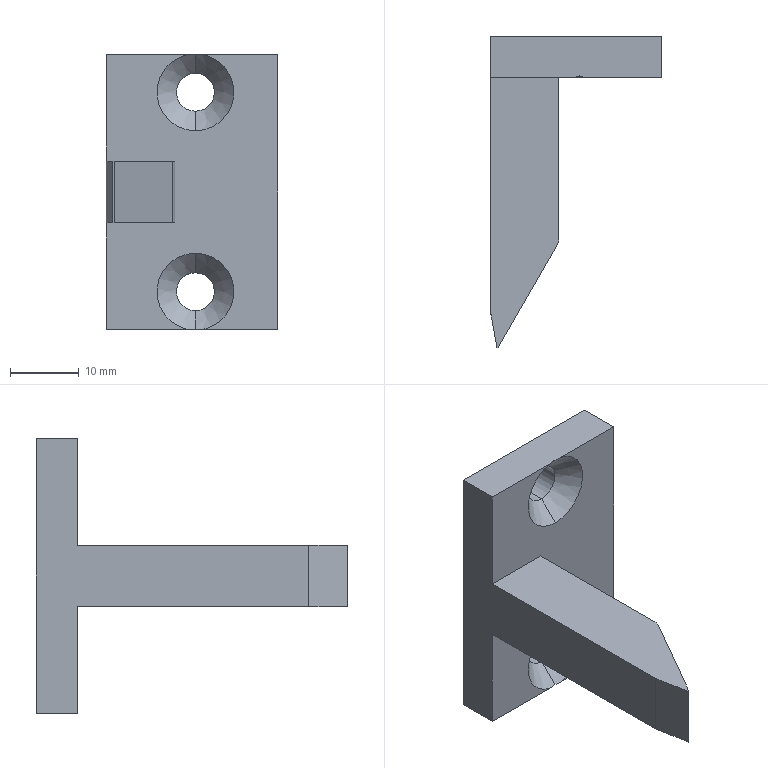Part | STEP file | PN_0002NACCTV wedge pin 527 | 1 solid | 21 faces | box 25 x 45.321 x 40 mm | volume 8429 mm3 | plane 12 | cylinder 5 | cone 4 | commonest cylinder face diameters 5.5 x4 4 x1
STEP:
#1=CARTESIAN_POINT('',(4.4,39.275,-11.75));
#2=VERTEX_POINT('',#1);
#3=CARTESIAN_POINT('',(4.4,39.275,-17.25));
#4=VERTEX_POINT('',#3);
#5=CARTESIAN_POINT('',(4.4,39.275,-14.5));
#6=DIRECTION('',(0.,-1.,0.));
#7=DIRECTION('',(0.,0.,-1.));
#8=AXIS2_PLACEMENT_3D('',#5,#6,#7);
#9=CIRCLE('',#8,2.75);
#10=EDGE_CURVE('',#2,#4,#9,.T.);
#11=ORIENTED_EDGE('',*,*,#10,.F.);
#12=CARTESIAN_POINT('',(4.4,36.425,-8.9));
#13=VERTEX_POINT('',#12);
#14=CARTESIAN_POINT('',(4.4,36.425,-8.9));
#15=DIRECTION('',(0.,-0.7071,0.7071));
#16=VECTOR('',#15,1000.);
#17=LINE('',#14,#16);
#18=EDGE_CURVE('',#2,#13,#17,.T.);
#19=ORIENTED_EDGE('',*,*,#18,.T.);
#20=CARTESIAN_POINT('',(3.346,36.425,-20.));
#21=VERTEX_POINT('',#20);
#22=CARTESIAN_POINT('',(4.4,36.425,-14.5));
#23=DIRECTION('',(0.,-1.,0.));
#24=DIRECTION('',(0.,0.,-1.));
#25=AXIS2_PLACEMENT_3D('',#22,#23,#24);
#26=CIRCLE('',#25,5.6);
#27=EDGE_CURVE('',#13,#21,#26,.T.);
#28=ORIENTED_EDGE('',*,*,#27,.T.);
#29=CARTESIAN_POINT('',(4.4,36.525,-20.));
#30=VERTEX_POINT('',#29);
#31=CARTESIAN_POINT('',(3.346,36.425,-20.));
#32=CARTESIAN_POINT('',(3.695,36.491,-20.));
#33=CARTESIAN_POINT('',(4.047,36.525,-20.));
#34=CARTESIAN_POINT('',(4.4,36.525,-20.));
#35=B_SPLINE_CURVE_WITH_KNOTS('',3,(#31,#32,#33,#34),.UNSPECIFIED.,.F.,.F.,(4,4),(0.01324,0.01428),.UNSPECIFIED.);
#36=EDGE_CURVE('',#21,#30,#35,.T.);
#37=ORIENTED_EDGE('',*,*,#36,.T.);
#38=CARTESIAN_POINT('',(4.4,36.425,-20.1));
#39=DIRECTION('',(0.,-0.7071,-0.7071));
#40=VECTOR('',#39,1000.);
#41=LINE('',#38,#40);
#42=EDGE_CURVE('',#4,#30,#41,.T.);
#43=ORIENTED_EDGE('',*,*,#42,.F.);
#44=EDGE_LOOP('',(#11,#19,#28,#37,#43));
#45=FACE_OUTER_BOUND('',#44,.T.);
#46=CARTESIAN_POINT('',(4.4,36.425,-14.5));
#47=DIRECTION('',(0.,-1.,0.));
#48=DIRECTION('',(0.,0.,-1.));
#49=AXIS2_PLACEMENT_3D('',#46,#47,#48);
#50=CONICAL_SURFACE('',#49,5.6,0.7854);
#51=ADVANCED_FACE('',(#45),#50,.F.);
#52=CARTESIAN_POINT('',(4.4,42.425,-11.75));
#53=VERTEX_POINT('',#52);
#54=CARTESIAN_POINT('',(4.4,42.425,-17.25));
#55=VERTEX_POINT('',#54);
#56=CARTESIAN_POINT('',(4.4,42.425,-14.5));
#57=DIRECTION('',(0.,-1.,0.));
#58=DIRECTION('',(0.,0.,-1.));
#59=AXIS2_PLACEMENT_3D('',#56,#57,#58);
#60=CIRCLE('',#59,2.75);
#61=EDGE_CURVE('',#53,#55,#60,.T.);
#62=ORIENTED_EDGE('',*,*,#61,.F.);
#63=CARTESIAN_POINT('',(4.4,36.425,-11.75));
#64=DIRECTION('',(0.,-1.,0.));
#65=VECTOR('',#64,1000.);
#66=LINE('',#63,#65);
#67=EDGE_CURVE('',#53,#2,#66,.T.);
#68=ORIENTED_EDGE('',*,*,#67,.T.);
#69=ORIENTED_EDGE('',*,*,#10,.T.);
#70=CARTESIAN_POINT('',(4.4,36.425,-17.25));
#71=DIRECTION('',(0.,-1.,0.));
#72=VECTOR('',#71,1000.);
#73=LINE('',#70,#72);
#74=EDGE_CURVE('',#55,#4,#73,.T.);
#75=ORIENTED_EDGE('',*,*,#74,.F.);
#76=EDGE_LOOP('',(#62,#68,#69,#75));
#77=FACE_OUTER_BOUND('',#76,.T.);
#78=CARTESIAN_POINT('',(4.4,36.425,-14.5));
#79=DIRECTION('',(0.,-1.,0.));
#80=DIRECTION('',(0.,0.,-1.));
#81=AXIS2_PLACEMENT_3D('',#78,#79,#80);
#82=CYLINDRICAL_SURFACE('',#81,2.75);
#83=ADVANCED_FACE('',(#77),#82,.F.);
#84=CARTESIAN_POINT('',(4.4,39.275,17.25));
#85=VERTEX_POINT('',#84);
#86=CARTESIAN_POINT('',(4.4,39.275,11.75));
#87=VERTEX_POINT('',#86);
#88=CARTESIAN_POINT('',(4.4,39.275,14.5));
#89=DIRECTION('',(0.,-1.,0.));
#90=DIRECTION('',(0.,0.,-1.));
#91=AXIS2_PLACEMENT_3D('',#88,#89,#90);
#92=CIRCLE('',#91,2.75);
#93=EDGE_CURVE('',#85,#87,#92,.T.);
#94=ORIENTED_EDGE('',*,*,#93,.F.);
#95=CARTESIAN_POINT('',(4.4,36.525,20.));
#96=VERTEX_POINT('',#95);
#97=CARTESIAN_POINT('',(4.4,36.425,20.1));
#98=DIRECTION('',(0.,-0.7071,0.7071));
#99=VECTOR('',#98,1000.);
#100=LINE('',#97,#99);
#101=EDGE_CURVE('',#85,#96,#100,.T.);
#102=ORIENTED_EDGE('',*,*,#101,.T.);
#103=CARTESIAN_POINT('',(3.346,36.425,20.));
#104=VERTEX_POINT('',#103);
#105=CARTESIAN_POINT('',(4.4,36.525,20.));
#106=CARTESIAN_POINT('',(4.047,36.525,20.));
#107=CARTESIAN_POINT('',(3.695,36.491,20.));
#108=CARTESIAN_POINT('',(3.346,36.425,20.));
#109=B_SPLINE_CURVE_WITH_KNOTS('',3,(#105,#106,#107,#108),.UNSPECIFIED.,.F.,.F.,(4,4),(0.007613,0.008661),.UNSPECIFIED.);
#110=EDGE_CURVE('',#96,#104,#109,.T.);
#111=ORIENTED_EDGE('',*,*,#110,.T.);
#112=CARTESIAN_POINT('',(4.4,36.425,8.9));
#113=VERTEX_POINT('',#112);
#114=CARTESIAN_POINT('',(4.4,36.425,14.5));
#115=DIRECTION('',(0.,-1.,0.));
#116=DIRECTION('',(0.,0.,-1.));
#117=AXIS2_PLACEMENT_3D('',#114,#115,#116);
#118=CIRCLE('',#117,5.6);
#119=EDGE_CURVE('',#104,#113,#118,.T.);
#120=ORIENTED_EDGE('',*,*,#119,.T.);
#121=CARTESIAN_POINT('',(4.4,36.425,8.9));
#122=DIRECTION('',(0.,-0.7071,-0.7071));
#123=VECTOR('',#122,1000.);
#124=LINE('',#121,#123);
#125=EDGE_CURVE('',#87,#113,#124,.T.);
#126=ORIENTED_EDGE('',*,*,#125,.F.);
#127=EDGE_LOOP('',(#94,#102,#111,#120,#126));
#128=FACE_OUTER_BOUND('',#127,.T.);
#129=CARTESIAN_POINT('',(4.4,36.425,14.5));
#130=DIRECTION('',(0.,-1.,0.));
#131=DIRECTION('',(0.,0.,-1.));
#132=AXIS2_PLACEMENT_3D('',#129,#130,#131);
#133=CONICAL_SURFACE('',#132,5.6,0.7854);
#134=ADVANCED_FACE('',(#128),#133,.F.);
#135=CARTESIAN_POINT('',(4.4,42.425,17.25));
#136=VERTEX_POINT('',#135);
#137=CARTESIAN_POINT('',(4.4,42.425,11.75));
#138=VERTEX_POINT('',#137);
#139=CARTESIAN_POINT('',(4.4,42.425,14.5));
#140=DIRECTION('',(0.,-1.,0.));
#141=DIRECTION('',(0.,0.,-1.));
#142=AXIS2_PLACEMENT_3D('',#139,#140,#141);
#143=CIRCLE('',#142,2.75);
#144=EDGE_CURVE('',#136,#138,#143,.T.);
#145=ORIENTED_EDGE('',*,*,#144,.F.);
#146=CARTESIAN_POINT('',(4.4,36.425,17.25));
#147=DIRECTION('',(0.,-1.,0.));
#148=VECTOR('',#147,1000.);
#149=LINE('',#146,#148);
#150=EDGE_CURVE('',#136,#85,#149,.T.);
#151=ORIENTED_EDGE('',*,*,#150,.T.);
#152=ORIENTED_EDGE('',*,*,#93,.T.);
#153=CARTESIAN_POINT('',(4.4,36.425,11.75));
#154=DIRECTION('',(0.,-1.,0.));
#155=VECTOR('',#154,1000.);
#156=LINE('',#153,#155);
#157=EDGE_CURVE('',#138,#87,#156,.T.);
#158=ORIENTED_EDGE('',*,*,#157,.F.);
#159=EDGE_LOOP('',(#145,#151,#152,#158));
#160=FACE_OUTER_BOUND('',#159,.T.);
#161=CARTESIAN_POINT('',(4.4,36.425,14.5));
#162=DIRECTION('',(0.,-1.,0.));
#163=DIRECTION('',(0.,0.,-1.));
#164=AXIS2_PLACEMENT_3D('',#161,#162,#163);
#165=CYLINDRICAL_SURFACE('',#164,2.75);
#166=ADVANCED_FACE('',(#160),#165,.F.);
#167=CARTESIAN_POINT('',(-8.6,42.425,20.));
#168=VERTEX_POINT('',#167);
#169=CARTESIAN_POINT('',(-8.6,42.425,-20.));
#170=VERTEX_POINT('',#169);
#171=CARTESIAN_POINT('',(-8.6,42.425,4.5));
#172=DIRECTION('',(0.,0.,-1.));
#173=VECTOR('',#172,1000.);
#174=LINE('',#171,#173);
#175=EDGE_CURVE('',#168,#170,#174,.T.);
#176=ORIENTED_EDGE('',*,*,#175,.T.);
#177=CARTESIAN_POINT('',(-8.6,36.425,-20.));
#178=VERTEX_POINT('',#177);
#179=CARTESIAN_POINT('',(-8.6,36.425,-20.));
#180=DIRECTION('',(0.,1.,0.));
#181=VECTOR('',#180,1000.);
#182=LINE('',#179,#181);
#183=EDGE_CURVE('',#178,#170,#182,.T.);
#184=ORIENTED_EDGE('',*,*,#183,.F.);
#185=CARTESIAN_POINT('',(-8.6,36.425,-4.5));
#186=VERTEX_POINT('',#185);
#187=CARTESIAN_POINT('',(-8.6,36.425,-20.));
#188=DIRECTION('',(0.,0.,1.));
#189=VECTOR('',#188,1000.);
#190=LINE('',#187,#189);
#191=EDGE_CURVE('',#178,#186,#190,.T.);
#192=ORIENTED_EDGE('',*,*,#191,.T.);
#193=CARTESIAN_POINT('',(-8.6,2.776,-4.5));
#194=VERTEX_POINT('',#193);
#195=CARTESIAN_POINT('',(-8.6,-4.896,-4.5));
#196=DIRECTION('',(0.,-1.,0.));
#197=VECTOR('',#196,1000.);
#198=LINE('',#195,#197);
#199=EDGE_CURVE('',#186,#194,#198,.T.);
#200=ORIENTED_EDGE('',*,*,#199,.T.);
#201=CARTESIAN_POINT('',(-8.6,2.776,4.5));
#202=VERTEX_POINT('',#201);
#203=CARTESIAN_POINT('',(-8.6,2.776,4.5));
#204=DIRECTION('',(0.,0.,1.));
#205=VECTOR('',#204,1000.);
#206=LINE('',#203,#205);
#207=EDGE_CURVE('',#194,#202,#206,.T.);
#208=ORIENTED_EDGE('',*,*,#207,.T.);
#209=CARTESIAN_POINT('',(-8.6,36.425,4.5));
#210=VERTEX_POINT('',#209);
#211=CARTESIAN_POINT('',(-8.6,-4.896,4.5));
#212=DIRECTION('',(0.,-1.,0.));
#213=VECTOR('',#212,1000.);
#214=LINE('',#211,#213);
#215=EDGE_CURVE('',#210,#202,#214,.T.);
#216=ORIENTED_EDGE('',*,*,#215,.F.);
#217=CARTESIAN_POINT('',(-8.6,36.425,20.));
#218=VERTEX_POINT('',#217);
#219=CARTESIAN_POINT('',(-8.6,36.425,4.5));
#220=DIRECTION('',(0.,0.,1.));
#221=VECTOR('',#220,1000.);
#222=LINE('',#219,#221);
#223=EDGE_CURVE('',#210,#218,#222,.T.);
#224=ORIENTED_EDGE('',*,*,#223,.T.);
#225=CARTESIAN_POINT('',(-8.6,36.425,20.));
#226=DIRECTION('',(0.,1.,0.));
#227=VECTOR('',#226,1000.);
#228=LINE('',#225,#227);
#229=EDGE_CURVE('',#218,#168,#228,.T.);
#230=ORIENTED_EDGE('',*,*,#229,.T.);
#231=EDGE_LOOP('',(#176,#184,#192,#200,#208,#216,#224,#230));
#232=FACE_OUTER_BOUND('',#231,.T.);
#233=CARTESIAN_POINT('',(-8.6,-4.896,4.5));
#234=DIRECTION('',(1.,0.,0.));
#235=DIRECTION('',(0.,0.,-1.));
#236=AXIS2_PLACEMENT_3D('',#233,#234,#235);
#237=PLANE('',#236);
#238=ADVANCED_FACE('',(#232),#237,.F.);
#239=CARTESIAN_POINT('',(-7.445,-2.896,-4.5));
#240=VERTEX_POINT('',#239);
#241=CARTESIAN_POINT('',(1.132,11.961,-4.5));
#242=VERTEX_POINT('',#241);
#243=CARTESIAN_POINT('',(-8.6,-4.896,-4.5));
#244=DIRECTION('',(0.5,0.866,0.));
#245=VECTOR('',#244,1000.);
#246=LINE('',#243,#245);
#247=EDGE_CURVE('',#240,#242,#246,.T.);
#248=ORIENTED_EDGE('',*,*,#247,.T.);
#249=CARTESIAN_POINT('',(1.132,11.961,4.5));
#250=VERTEX_POINT('',#249);
#251=CARTESIAN_POINT('',(1.132,11.961,4.5));
#252=DIRECTION('',(0.,0.,1.));
#253=VECTOR('',#252,1000.);
#254=LINE('',#251,#253);
#255=EDGE_CURVE('',#242,#250,#254,.T.);
#256=ORIENTED_EDGE('',*,*,#255,.T.);
#257=CARTESIAN_POINT('',(-7.445,-2.896,4.5));
#258=VERTEX_POINT('',#257);
#259=CARTESIAN_POINT('',(-8.6,-4.896,4.5));
#260=DIRECTION('',(0.5,0.866,0.));
#261=VECTOR('',#260,1000.);
#262=LINE('',#259,#261);
#263=EDGE_CURVE('',#258,#250,#262,.T.);
#264=ORIENTED_EDGE('',*,*,#263,.F.);
#265=CARTESIAN_POINT('',(-7.445,-2.896,-4.5));
#266=DIRECTION('',(0.,0.,1.));
#267=VECTOR('',#266,1000.);
#268=LINE('',#265,#267);
#269=EDGE_CURVE('',#240,#258,#268,.T.);
#270=ORIENTED_EDGE('',*,*,#269,.F.);
#271=EDGE_LOOP('',(#248,#256,#264,#270));
#272=FACE_OUTER_BOUND('',#271,.T.);
#273=CARTESIAN_POINT('',(-8.6,-4.896,4.5));
#274=DIRECTION('',(-0.866,0.5,0.));
#275=DIRECTION('',(-0.5,-0.866,0.));
#276=AXIS2_PLACEMENT_3D('',#273,#274,#275);
#277=PLANE('',#276);
#278=ADVANCED_FACE('',(#272),#277,.F.);
#279=CARTESIAN_POINT('',(1.4,12.961,-4.5));
#280=VERTEX_POINT('',#279);
#281=CARTESIAN_POINT('',(1.4,36.425,-4.5));
#282=VERTEX_POINT('',#281);
#283=CARTESIAN_POINT('',(1.4,42.425,-4.5));
#284=DIRECTION('',(0.,1.,0.));
#285=VECTOR('',#284,1000.);
#286=LINE('',#283,#285);
#287=EDGE_CURVE('',#280,#282,#286,.T.);
#288=ORIENTED_EDGE('',*,*,#287,.T.);
#289=CARTESIAN_POINT('',(1.4,36.425,4.5));
#290=VERTEX_POINT('',#289);
#291=CARTESIAN_POINT('',(1.4,36.425,-4.5));
#292=DIRECTION('',(0.,0.,1.));
#293=VECTOR('',#292,1000.);
#294=LINE('',#291,#293);
#295=EDGE_CURVE('',#282,#290,#294,.T.);
#296=ORIENTED_EDGE('',*,*,#295,.T.);
#297=CARTESIAN_POINT('',(1.4,12.961,4.5));
#298=VERTEX_POINT('',#297);
#299=CARTESIAN_POINT('',(1.4,42.425,4.5));
#300=DIRECTION('',(0.,1.,0.));
#301=VECTOR('',#300,1000.);
#302=LINE('',#299,#301);
#303=EDGE_CURVE('',#298,#290,#302,.T.);
#304=ORIENTED_EDGE('',*,*,#303,.F.);
#305=CARTESIAN_POINT('',(1.4,12.961,4.5));
#306=DIRECTION('',(0.,0.,-1.));
#307=VECTOR('',#306,1000.);
#308=LINE('',#305,#307);
#309=EDGE_CURVE('',#298,#280,#308,.T.);
#310=ORIENTED_EDGE('',*,*,#309,.T.);
#311=EDGE_LOOP('',(#288,#296,#304,#310));
#312=FACE_OUTER_BOUND('',#311,.T.);
#313=CARTESIAN_POINT('',(1.4,42.425,4.5));
#314=DIRECTION('',(-1.,0.,0.));
#315=DIRECTION('',(0.,-1.,0.));
#316=AXIS2_PLACEMENT_3D('',#313,#314,#315);
#317=PLANE('',#316);
#318=ADVANCED_FACE('',(#312),#317,.F.);
#319=CARTESIAN_POINT('',(4.4,42.425,-14.5));
#320=DIRECTION('',(0.,-1.,0.));
#321=DIRECTION('',(0.,0.,-1.));
#322=AXIS2_PLACEMENT_3D('',#319,#320,#321);
#323=CIRCLE('',#322,2.75);
#324=EDGE_CURVE('',#55,#53,#323,.T.);
#325=ORIENTED_EDGE('',*,*,#324,.T.);
#326=ORIENTED_EDGE('',*,*,#61,.T.);
#327=EDGE_LOOP('',(#325,#326));
#328=FACE_BOUND('',#327,.T.);
#329=CARTESIAN_POINT('',(4.4,42.425,14.5));
#330=DIRECTION('',(0.,-1.,0.));
#331=DIRECTION('',(0.,0.,-1.));
#332=AXIS2_PLACEMENT_3D('',#329,#330,#331);
#333=CIRCLE('',#332,2.75);
#334=EDGE_CURVE('',#138,#136,#333,.T.);
#335=ORIENTED_EDGE('',*,*,#334,.T.);
#336=ORIENTED_EDGE('',*,*,#144,.T.);
#337=EDGE_LOOP('',(#335,#336));
#338=FACE_BOUND('',#337,.T.);
#339=ORIENTED_EDGE('',*,*,#175,.F.);
#340=CARTESIAN_POINT('',(16.4,42.425,20.));
#341=VERTEX_POINT('',#340);
#342=CARTESIAN_POINT('',(16.4,42.425,20.));
#343=DIRECTION('',(1.,0.,0.));
#344=VECTOR('',#343,1000.);
#345=LINE('',#342,#344);
#346=EDGE_CURVE('',#168,#341,#345,.T.);
#347=ORIENTED_EDGE('',*,*,#346,.T.);
#348=CARTESIAN_POINT('',(16.4,42.425,-20.));
#349=VERTEX_POINT('',#348);
#350=CARTESIAN_POINT('',(16.4,42.425,-20.));
#351=DIRECTION('',(0.,0.,-1.));
#352=VECTOR('',#351,1000.);
#353=LINE('',#350,#352);
#354=EDGE_CURVE('',#341,#349,#353,.T.);
#355=ORIENTED_EDGE('',*,*,#354,.T.);
#356=CARTESIAN_POINT('',(16.4,42.425,-20.));
#357=DIRECTION('',(-1.,0.,0.));
#358=VECTOR('',#357,1000.);
#359=LINE('',#356,#358);
#360=EDGE_CURVE('',#349,#170,#359,.T.);
#361=ORIENTED_EDGE('',*,*,#360,.T.);
#362=EDGE_LOOP('',(#339,#347,#355,#361));
#363=FACE_OUTER_BOUND('',#362,.T.);
#364=CARTESIAN_POINT('',(-8.6,42.425,4.5));
#365=DIRECTION('',(0.,-1.,0.));
#366=DIRECTION('',(0.,0.,-1.));
#367=AXIS2_PLACEMENT_3D('',#364,#365,#366);
#368=PLANE('',#367);
#369=ADVANCED_FACE('',(#328,#338,#363),#368,.F.);
#370=ORIENTED_EDGE('',*,*,#303,.T.);
#371=CARTESIAN_POINT('',(1.4,36.425,4.5));
#372=DIRECTION('',(-1.,0.,0.));
#373=VECTOR('',#372,1000.);
#374=LINE('',#371,#373);
#375=EDGE_CURVE('',#290,#210,#374,.T.);
#376=ORIENTED_EDGE('',*,*,#375,.T.);
#377=ORIENTED_EDGE('',*,*,#215,.T.);
#378=CARTESIAN_POINT('',(-7.6,-2.896,4.5));
#379=VERTEX_POINT('',#378);
#380=CARTESIAN_POINT('',(-8.6,2.776,4.5));
#381=DIRECTION('',(0.1736,-0.9848,0.));
#382=VECTOR('',#381,1000.);
#383=LINE('',#380,#382);
#384=EDGE_CURVE('',#202,#379,#383,.T.);
#385=ORIENTED_EDGE('',*,*,#384,.T.);
#386=CARTESIAN_POINT('',(-8.6,-2.896,4.5));
#387=DIRECTION('',(-1.,0.,0.));
#388=VECTOR('',#387,1000.);
#389=LINE('',#386,#388);
#390=EDGE_CURVE('',#258,#379,#389,.T.);
#391=ORIENTED_EDGE('',*,*,#390,.F.);
#392=ORIENTED_EDGE('',*,*,#263,.T.);
#393=CARTESIAN_POINT('',(-0.6,12.961,4.5));
#394=DIRECTION('',(0.,0.,1.));
#395=DIRECTION('',(-1.,0.,0.));
#396=AXIS2_PLACEMENT_3D('',#393,#394,#395);
#397=CIRCLE('',#396,2.);
#398=EDGE_CURVE('',#250,#298,#397,.T.);
#399=ORIENTED_EDGE('',*,*,#398,.T.);
#400=EDGE_LOOP('',(#370,#376,#377,#385,#391,#392,#399));
#401=FACE_OUTER_BOUND('',#400,.T.);
#402=CARTESIAN_POINT('',(0.,0.,4.5));
#403=DIRECTION('',(0.,0.,-1.));
#404=DIRECTION('',(-1.,0.,0.));
#405=AXIS2_PLACEMENT_3D('',#402,#403,#404);
#406=PLANE('',#405);
#407=ADVANCED_FACE('',(#401),#406,.F.);
#408=CARTESIAN_POINT('',(1.4,36.425,-4.5));
#409=DIRECTION('',(1.,0.,0.));
#410=VECTOR('',#409,1000.);
#411=LINE('',#408,#410);
#412=EDGE_CURVE('',#186,#282,#411,.T.);
#413=ORIENTED_EDGE('',*,*,#412,.T.);
#414=ORIENTED_EDGE('',*,*,#287,.F.);
#415=CARTESIAN_POINT('',(-0.6,12.961,-4.5));
#416=DIRECTION('',(0.,0.,-1.));
#417=DIRECTION('',(-1.,0.,0.));
#418=AXIS2_PLACEMENT_3D('',#415,#416,#417);
#419=CIRCLE('',#418,2.);
#420=EDGE_CURVE('',#280,#242,#419,.T.);
#421=ORIENTED_EDGE('',*,*,#420,.T.);
#422=ORIENTED_EDGE('',*,*,#247,.F.);
#423=CARTESIAN_POINT('',(-7.6,-2.896,-4.5));
#424=VERTEX_POINT('',#423);
#425=CARTESIAN_POINT('',(-8.6,-2.896,-4.5));
#426=DIRECTION('',(-1.,0.,0.));
#427=VECTOR('',#426,1000.);
#428=LINE('',#425,#427);
#429=EDGE_CURVE('',#240,#424,#428,.T.);
#430=ORIENTED_EDGE('',*,*,#429,.T.);
#431=CARTESIAN_POINT('',(-7.866,-1.387,-4.5));
#432=DIRECTION('',(-0.1736,0.9848,0.));
#433=VECTOR('',#432,1000.);
#434=LINE('',#431,#433);
#435=EDGE_CURVE('',#424,#194,#434,.T.);
#436=ORIENTED_EDGE('',*,*,#435,.T.);
#437=ORIENTED_EDGE('',*,*,#199,.F.);
#438=EDGE_LOOP('',(#413,#414,#421,#422,#430,#436,#437));
#439=FACE_OUTER_BOUND('',#438,.T.);
#440=CARTESIAN_POINT('',(0.,0.,-4.5));
#441=DIRECTION('',(0.,0.,-1.));
#442=DIRECTION('',(-1.,0.,0.));
#443=AXIS2_PLACEMENT_3D('',#440,#441,#442);
#444=PLANE('',#443);
#445=ADVANCED_FACE('',(#439),#444,.T.);
#446=ORIENTED_EDGE('',*,*,#390,.T.);
#447=CARTESIAN_POINT('',(-7.6,-2.896,-4.5));
#448=DIRECTION('',(0.,0.,-1.));
#449=VECTOR('',#448,1000.);
#450=LINE('',#447,#449);
#451=EDGE_CURVE('',#379,#424,#450,.T.);
#452=ORIENTED_EDGE('',*,*,#451,.T.);
#453=ORIENTED_EDGE('',*,*,#429,.F.);
#454=ORIENTED_EDGE('',*,*,#269,.T.);
#455=EDGE_LOOP('',(#446,#452,#453,#454));
#456=FACE_OUTER_BOUND('',#455,.T.);
#457=CARTESIAN_POINT('',(-8.6,-2.896,-4.5));
#458=DIRECTION('',(0.,1.,0.));
#459=DIRECTION('',(-1.,0.,0.));
#460=AXIS2_PLACEMENT_3D('',#457,#458,#459);
#461=PLANE('',#460);
#462=ADVANCED_FACE('',(#456),#461,.F.);
#463=ORIENTED_EDGE('',*,*,#398,.F.);
#464=ORIENTED_EDGE('',*,*,#255,.F.);
#465=ORIENTED_EDGE('',*,*,#420,.F.);
#466=ORIENTED_EDGE('',*,*,#309,.F.);
#467=EDGE_LOOP('',(#463,#464,#465,#466));
#468=FACE_OUTER_BOUND('',#467,.T.);
#469=CARTESIAN_POINT('',(-0.6,12.961,4.5));
#470=DIRECTION('',(0.,0.,-1.));
#471=DIRECTION('',(-1.,0.,0.));
#472=AXIS2_PLACEMENT_3D('',#469,#470,#471);
#473=CYLINDRICAL_SURFACE('',#472,2.);
#474=ADVANCED_FACE('',(#468),#473,.T.);
#475=ORIENTED_EDGE('',*,*,#435,.F.);
#476=ORIENTED_EDGE('',*,*,#451,.F.);
#477=ORIENTED_EDGE('',*,*,#384,.F.);
#478=ORIENTED_EDGE('',*,*,#207,.F.);
#479=EDGE_LOOP('',(#475,#476,#477,#478));
#480=FACE_OUTER_BOUND('',#479,.T.);
#481=CARTESIAN_POINT('',(-8.6,2.776,4.5));
#482=DIRECTION('',(0.9848,0.1736,0.));
#483=DIRECTION('',(0.,0.,1.));
#484=AXIS2_PLACEMENT_3D('',#481,#482,#483);
#485=PLANE('',#484);
#486=ADVANCED_FACE('',(#480),#485,.F.);
#487=ORIENTED_EDGE('',*,*,#354,.F.);
#488=CARTESIAN_POINT('',(16.4,36.425,20.));
#489=VERTEX_POINT('',#488);
#490=CARTESIAN_POINT('',(16.4,36.425,20.));
#491=DIRECTION('',(0.,1.,0.));
#492=VECTOR('',#491,1000.);
#493=LINE('',#490,#492);
#494=EDGE_CURVE('',#489,#341,#493,.T.);
#495=ORIENTED_EDGE('',*,*,#494,.F.);
#496=CARTESIAN_POINT('',(16.4,36.425,-20.));
#497=VERTEX_POINT('',#496);
#498=CARTESIAN_POINT('',(16.4,36.425,-20.));
#499=DIRECTION('',(0.,0.,-1.));
#500=VECTOR('',#499,1000.);
#501=LINE('',#498,#500);
#502=EDGE_CURVE('',#489,#497,#501,.T.);
#503=ORIENTED_EDGE('',*,*,#502,.T.);
#504=CARTESIAN_POINT('',(16.4,36.425,-20.));
#505=DIRECTION('',(0.,1.,0.));
#506=VECTOR('',#505,1000.);
#507=LINE('',#504,#506);
#508=EDGE_CURVE('',#497,#349,#507,.T.);
#509=ORIENTED_EDGE('',*,*,#508,.T.);
#510=EDGE_LOOP('',(#487,#495,#503,#509));
#511=FACE_OUTER_BOUND('',#510,.T.);
#512=CARTESIAN_POINT('',(16.4,36.425,-20.));
#513=DIRECTION('',(1.,0.,0.));
#514=DIRECTION('',(0.,0.,-1.));
#515=AXIS2_PLACEMENT_3D('',#512,#513,#514);
#516=PLANE('',#515);
#517=ADVANCED_FACE('',(#511),#516,.T.);
#518=CARTESIAN_POINT('',(5.454,36.425,20.));
#519=VERTEX_POINT('',#518);
#520=CARTESIAN_POINT('',(5.454,36.425,20.));
#521=CARTESIAN_POINT('',(5.108,36.49,20.));
#522=CARTESIAN_POINT('',(4.752,36.525,20.));
#523=CARTESIAN_POINT('',(4.4,36.525,20.));
#524=B_SPLINE_CURVE_WITH_KNOTS('',3,(#520,#521,#522,#523),.UNSPECIFIED.,.F.,.F.,(4,4),(0.006568,0.007613),.UNSPECIFIED.);
#525=EDGE_CURVE('',#519,#96,#524,.T.);
#526=ORIENTED_EDGE('',*,*,#525,.F.);
#527=CARTESIAN_POINT('',(16.4,36.425,20.));
#528=DIRECTION('',(1.,0.,0.));
#529=VECTOR('',#528,1000.);
#530=LINE('',#527,#529);
#531=EDGE_CURVE('',#519,#489,#530,.T.);
#532=ORIENTED_EDGE('',*,*,#531,.T.);
#533=ORIENTED_EDGE('',*,*,#494,.T.);
#534=ORIENTED_EDGE('',*,*,#346,.F.);
#535=ORIENTED_EDGE('',*,*,#229,.F.);
#536=CARTESIAN_POINT('',(16.4,36.425,20.));
#537=DIRECTION('',(1.,0.,0.));
#538=VECTOR('',#537,1000.);
#539=LINE('',#536,#538);
#540=EDGE_CURVE('',#218,#104,#539,.T.);
#541=ORIENTED_EDGE('',*,*,#540,.T.);
#542=ORIENTED_EDGE('',*,*,#110,.F.);
#543=EDGE_LOOP('',(#526,#532,#533,#534,#535,#541,#542));
#544=FACE_OUTER_BOUND('',#543,.T.);
#545=CARTESIAN_POINT('',(16.4,36.425,20.));
#546=DIRECTION('',(0.,0.,1.));
#547=DIRECTION('',(1.,0.,0.));
#548=AXIS2_PLACEMENT_3D('',#545,#546,#547);
#549=PLANE('',#548);
#550=ADVANCED_FACE('',(#544),#549,.T.);
#551=ORIENTED_EDGE('',*,*,#36,.F.);
#552=CARTESIAN_POINT('',(16.4,36.425,-20.));
#553=DIRECTION('',(-1.,0.,0.));
#554=VECTOR('',#553,1000.);
#555=LINE('',#552,#554);
#556=EDGE_CURVE('',#21,#178,#555,.T.);
#557=ORIENTED_EDGE('',*,*,#556,.T.);
#558=ORIENTED_EDGE('',*,*,#183,.T.);
#559=ORIENTED_EDGE('',*,*,#360,.F.);
#560=ORIENTED_EDGE('',*,*,#508,.F.);
#561=CARTESIAN_POINT('',(5.454,36.425,-20.));
#562=VERTEX_POINT('',#561);
#563=CARTESIAN_POINT('',(16.4,36.425,-20.));
#564=DIRECTION('',(-1.,0.,0.));
#565=VECTOR('',#564,1000.);
#566=LINE('',#563,#565);
#567=EDGE_CURVE('',#497,#562,#566,.T.);
#568=ORIENTED_EDGE('',*,*,#567,.T.);
#569=CARTESIAN_POINT('',(4.4,36.525,-20.));
#570=CARTESIAN_POINT('',(4.752,36.525,-20.));
#571=CARTESIAN_POINT('',(5.108,36.49,-20.));
#572=CARTESIAN_POINT('',(5.454,36.425,-20.));
#573=B_SPLINE_CURVE_WITH_KNOTS('',3,(#569,#570,#571,#572),.UNSPECIFIED.,.F.,.F.,(4,4),(0.01428,0.01532),.UNSPECIFIED.);
#574=EDGE_CURVE('',#30,#562,#573,.T.);
#575=ORIENTED_EDGE('',*,*,#574,.F.);
#576=EDGE_LOOP('',(#551,#557,#558,#559,#560,#568,#575));
#577=FACE_OUTER_BOUND('',#576,.T.);
#578=CARTESIAN_POINT('',(16.4,36.425,-20.));
#579=DIRECTION('',(0.,0.,-1.));
#580=DIRECTION('',(-1.,0.,0.));
#581=AXIS2_PLACEMENT_3D('',#578,#579,#580);
#582=PLANE('',#581);
#583=ADVANCED_FACE('',(#577),#582,.T.);
#584=CARTESIAN_POINT('',(4.4,36.425,-14.5));
#585=DIRECTION('',(0.,-1.,0.));
#586=DIRECTION('',(0.,0.,-1.));
#587=AXIS2_PLACEMENT_3D('',#584,#585,#586);
#588=CIRCLE('',#587,5.6);
#589=EDGE_CURVE('',#562,#13,#588,.T.);
#590=ORIENTED_EDGE('',*,*,#589,.F.);
#591=ORIENTED_EDGE('',*,*,#567,.F.);
#592=ORIENTED_EDGE('',*,*,#502,.F.);
#593=ORIENTED_EDGE('',*,*,#531,.F.);
#594=CARTESIAN_POINT('',(4.4,36.425,14.5));
#595=DIRECTION('',(0.,-1.,0.));
#596=DIRECTION('',(0.,0.,-1.));
#597=AXIS2_PLACEMENT_3D('',#594,#595,#596);
#598=CIRCLE('',#597,5.6);
#599=EDGE_CURVE('',#113,#519,#598,.T.);
#600=ORIENTED_EDGE('',*,*,#599,.F.);
#601=ORIENTED_EDGE('',*,*,#119,.F.);
#602=ORIENTED_EDGE('',*,*,#540,.F.);
#603=ORIENTED_EDGE('',*,*,#223,.F.);
#604=ORIENTED_EDGE('',*,*,#375,.F.);
#605=ORIENTED_EDGE('',*,*,#295,.F.);
#606=ORIENTED_EDGE('',*,*,#412,.F.);
#607=ORIENTED_EDGE('',*,*,#191,.F.);
#608=ORIENTED_EDGE('',*,*,#556,.F.);
#609=ORIENTED_EDGE('',*,*,#27,.F.);
#610=EDGE_LOOP('',(#590,#591,#592,#593,#600,#601,#602,#603,#604,#605,#606,#607,#608,#609));
#611=FACE_OUTER_BOUND('',#610,.T.);
#612=CARTESIAN_POINT('',(0.,36.425,0.));
#613=DIRECTION('',(0.,-1.,0.));
#614=DIRECTION('',(0.,0.,-1.));
#615=AXIS2_PLACEMENT_3D('',#612,#613,#614);
#616=PLANE('',#615);
#617=ADVANCED_FACE('',(#611),#616,.T.);
#618=ORIENTED_EDGE('',*,*,#150,.F.);
#619=ORIENTED_EDGE('',*,*,#334,.F.);
#620=ORIENTED_EDGE('',*,*,#157,.T.);
#621=CARTESIAN_POINT('',(4.4,39.275,14.5));
#622=DIRECTION('',(0.,-1.,0.));
#623=DIRECTION('',(0.,0.,-1.));
#624=AXIS2_PLACEMENT_3D('',#621,#622,#623);
#625=CIRCLE('',#624,2.75);
#626=EDGE_CURVE('',#87,#85,#625,.T.);
#627=ORIENTED_EDGE('',*,*,#626,.T.);
#628=EDGE_LOOP('',(#618,#619,#620,#627));
#629=FACE_OUTER_BOUND('',#628,.T.);
#630=CARTESIAN_POINT('',(4.4,36.425,14.5));
#631=DIRECTION('',(0.,-1.,0.));
#632=DIRECTION('',(0.,0.,-1.));
#633=AXIS2_PLACEMENT_3D('',#630,#631,#632);
#634=CYLINDRICAL_SURFACE('',#633,2.75);
#635=ADVANCED_FACE('',(#629),#634,.F.);
#636=ORIENTED_EDGE('',*,*,#101,.F.);
#637=ORIENTED_EDGE('',*,*,#626,.F.);
#638=ORIENTED_EDGE('',*,*,#125,.T.);
#639=ORIENTED_EDGE('',*,*,#599,.T.);
#640=ORIENTED_EDGE('',*,*,#525,.T.);
#641=EDGE_LOOP('',(#636,#637,#638,#639,#640));
#642=FACE_OUTER_BOUND('',#641,.T.);
#643=CARTESIAN_POINT('',(4.4,36.425,14.5));
#644=DIRECTION('',(0.,-1.,0.));
#645=DIRECTION('',(0.,0.,-1.));
#646=AXIS2_PLACEMENT_3D('',#643,#644,#645);
#647=CONICAL_SURFACE('',#646,5.6,0.7854);
#648=ADVANCED_FACE('',(#642),#647,.F.);
#649=ORIENTED_EDGE('',*,*,#67,.F.);
#650=ORIENTED_EDGE('',*,*,#324,.F.);
#651=ORIENTED_EDGE('',*,*,#74,.T.);
#652=CARTESIAN_POINT('',(4.4,39.275,-14.5));
#653=DIRECTION('',(0.,-1.,0.));
#654=DIRECTION('',(0.,0.,-1.));
#655=AXIS2_PLACEMENT_3D('',#652,#653,#654);
#656=CIRCLE('',#655,2.75);
#657=EDGE_CURVE('',#4,#2,#656,.T.);
#658=ORIENTED_EDGE('',*,*,#657,.T.);
#659=EDGE_LOOP('',(#649,#650,#651,#658));
#660=FACE_OUTER_BOUND('',#659,.T.);
#661=CARTESIAN_POINT('',(4.4,36.425,-14.5));
#662=DIRECTION('',(0.,-1.,0.));
#663=DIRECTION('',(0.,0.,-1.));
#664=AXIS2_PLACEMENT_3D('',#661,#662,#663);
#665=CYLINDRICAL_SURFACE('',#664,2.75);
#666=ADVANCED_FACE('',(#660),#665,.F.);
#667=ORIENTED_EDGE('',*,*,#18,.F.);
#668=ORIENTED_EDGE('',*,*,#657,.F.);
#669=ORIENTED_EDGE('',*,*,#42,.T.);
#670=ORIENTED_EDGE('',*,*,#574,.T.);
#671=ORIENTED_EDGE('',*,*,#589,.T.);
#672=EDGE_LOOP('',(#667,#668,#669,#670,#671));
#673=FACE_OUTER_BOUND('',#672,.T.);
#674=CARTESIAN_POINT('',(4.4,36.425,-14.5));
#675=DIRECTION('',(0.,-1.,0.));
#676=DIRECTION('',(0.,0.,-1.));
#677=AXIS2_PLACEMENT_3D('',#674,#675,#676);
#678=CONICAL_SURFACE('',#677,5.6,0.7854);
#679=ADVANCED_FACE('',(#673),#678,.F.);
#680=CLOSED_SHELL('',(#51,#83,#134,#166,#238,#278,#318,#369,#407,#445,#462,#474,#486,#517,#550,#583,#617,#635,#648,#666,#679));
#681=MANIFOLD_SOLID_BREP('',#680);
#682=CARTESIAN_POINT('',(0.,0.,0.));
#683=DIRECTION('',(0.,0.,1.));
#684=DIRECTION('',(1.,0.,0.));
#685=AXIS2_PLACEMENT_3D('',#682,#683,#684);
#686=(LENGTH_UNIT()NAMED_UNIT(*)SI_UNIT(.MILLI.,.METRE.));
#687=UNCERTAINTY_MEASURE_WITH_UNIT(LENGTH_MEASURE(0.00001),#686,'','');
#688=(NAMED_UNIT(*)PLANE_ANGLE_UNIT()SI_UNIT($,.RADIAN.));
#689=(NAMED_UNIT(*)SI_UNIT($,.STERADIAN.)SOLID_ANGLE_UNIT());
#690=(GEOMETRIC_REPRESENTATION_CONTEXT(3)GLOBAL_UNCERTAINTY_ASSIGNED_CONTEXT((#687))GLOBAL_UNIT_ASSIGNED_CONTEXT((#686,#688,#689))REPRESENTATION_CONTEXT('',''));
#691=ADVANCED_BREP_SHAPE_REPRESENTATION('',(#681,#685),#690);